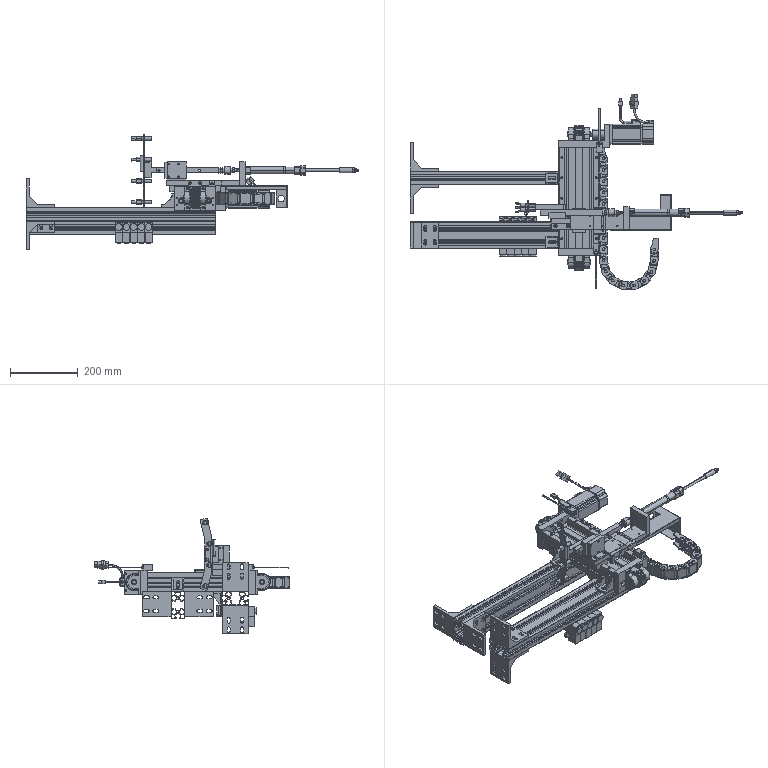Part | 80 solids | 6858 faces | volume 4123611 mm3 | plane 3761 | cylinder 2556 | spline 293 | cone 219 | torus 15 | sphere 14 | commonest cylinder face diameters 2 x314 1 x184 0.6 x154 0.96 x140 23.26 x119 9 x105